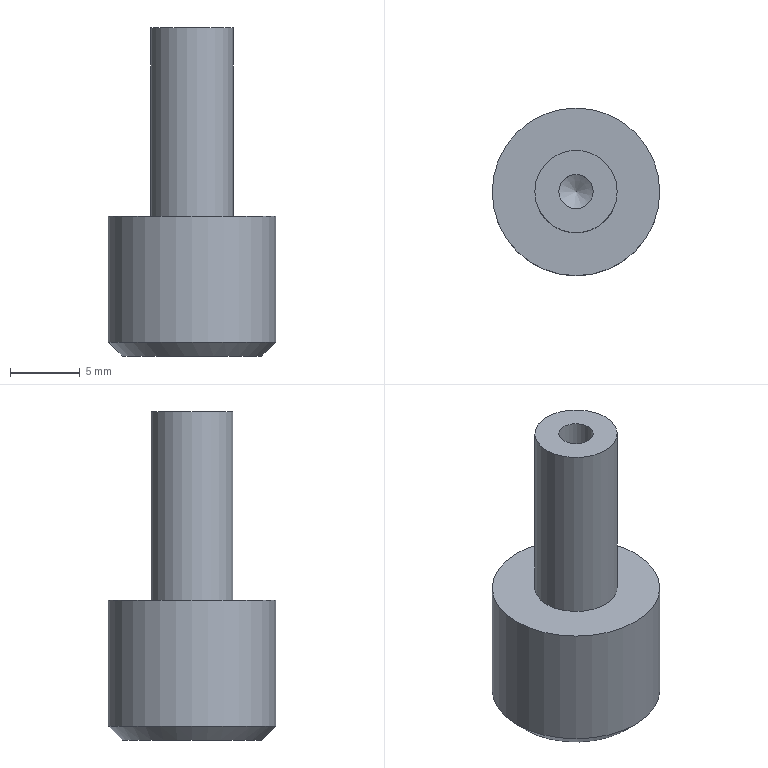Part | STEP file | 1-S938U-100524-007 | 1 solid | 10 faces | box 12 x 12 x 23.5 mm | volume 1339 mm3 | cylinder 4 | cone 3 | plane 3 | commonest cylinder face diameters 2.459 x1 3.242 x1 5.9 x1 12 x1
STEP:
#1=CARTESIAN_POINT('',(-6.,0.,1.));
#2=VERTEX_POINT('',#1);
#3=CARTESIAN_POINT('',(6.,0.,1.));
#4=VERTEX_POINT('',#3);
#5=CARTESIAN_POINT('',(0.,0.,1.));
#6=DIRECTION('',(0.,0.,-1.));
#7=DIRECTION('',(-1.,0.,0.));
#8=AXIS2_PLACEMENT_3D('',#5,#6,#7);
#9=CIRCLE('',#8,6.);
#10=EDGE_CURVE('',#2,#4,#9,.T.);
#11=ORIENTED_EDGE('',*,*,#10,.T.);
#12=CARTESIAN_POINT('',(5.,0.,0.));
#13=VERTEX_POINT('',#12);
#14=CARTESIAN_POINT('',(5.5,0.,0.5));
#15=DIRECTION('',(-0.7071,0.,-0.7071));
#16=VECTOR('',#15,5.5);
#17=LINE('',#14,#16);
#18=EDGE_CURVE('',#4,#13,#17,.T.);
#19=ORIENTED_EDGE('',*,*,#18,.T.);
#20=CARTESIAN_POINT('',(0.,0.,0.));
#21=DIRECTION('',(0.,0.,1.));
#22=DIRECTION('',(-1.,0.,0.));
#23=AXIS2_PLACEMENT_3D('',#20,#21,#22);
#24=CIRCLE('',#23,5.);
#25=EDGE_CURVE('',#13,#13,#24,.T.);
#26=ORIENTED_EDGE('',*,*,#25,.T.);
#27=ORIENTED_EDGE('',*,*,#18,.F.);
#28=CARTESIAN_POINT('',(0.,0.,1.));
#29=DIRECTION('',(0.,0.,-1.));
#30=DIRECTION('',(-1.,0.,0.));
#31=AXIS2_PLACEMENT_3D('',#28,#29,#30);
#32=CIRCLE('',#31,6.);
#33=EDGE_CURVE('',#4,#2,#32,.T.);
#34=ORIENTED_EDGE('',*,*,#33,.T.);
#35=EDGE_LOOP('',(#11,#19,#26,#27,#34));
#36=FACE_OUTER_BOUND('',#35,.T.);
#37=CARTESIAN_POINT('',(0.,0.,0.5));
#38=DIRECTION('',(0.,0.,1.));
#39=DIRECTION('',(-1.,0.,0.));
#40=AXIS2_PLACEMENT_3D('',#37,#38,#39);
#41=CONICAL_SURFACE('',#40,5.5,0.7854);
#42=ADVANCED_FACE('',(#36),#41,.T.);
#43=CARTESIAN_POINT('',(6.,0.,10.));
#44=VERTEX_POINT('',#43);
#45=CARTESIAN_POINT('',(-6.,0.,10.));
#46=VERTEX_POINT('',#45);
#47=CARTESIAN_POINT('',(0.,0.,10.));
#48=DIRECTION('',(0.,0.,1.));
#49=DIRECTION('',(1.,0.,0.));
#50=AXIS2_PLACEMENT_3D('',#47,#48,#49);
#51=CIRCLE('',#50,6.);
#52=EDGE_CURVE('',#44,#46,#51,.T.);
#53=ORIENTED_EDGE('',*,*,#52,.F.);
#54=CARTESIAN_POINT('',(0.,0.,10.));
#55=DIRECTION('',(0.,0.,1.));
#56=DIRECTION('',(1.,0.,0.));
#57=AXIS2_PLACEMENT_3D('',#54,#55,#56);
#58=CIRCLE('',#57,6.);
#59=EDGE_CURVE('',#46,#44,#58,.T.);
#60=ORIENTED_EDGE('',*,*,#59,.F.);
#61=CARTESIAN_POINT('',(-6.,0.,0.));
#62=DIRECTION('',(0.,0.,-1.));
#63=VECTOR('',#62,6.);
#64=LINE('',#61,#63);
#65=EDGE_CURVE('',#46,#2,#64,.T.);
#66=ORIENTED_EDGE('',*,*,#65,.T.);
#67=ORIENTED_EDGE('',*,*,#33,.F.);
#68=ORIENTED_EDGE('',*,*,#10,.F.);
#69=ORIENTED_EDGE('',*,*,#65,.F.);
#70=EDGE_LOOP('',(#53,#60,#66,#67,#68,#69));
#71=FACE_OUTER_BOUND('',#70,.T.);
#72=CARTESIAN_POINT('',(0.,0.,0.));
#73=DIRECTION('',(0.,0.,1.));
#74=DIRECTION('',(1.,0.,0.));
#75=AXIS2_PLACEMENT_3D('',#72,#73,#74);
#76=CYLINDRICAL_SURFACE('',#75,6.);
#77=ADVANCED_FACE('',(#71),#76,.T.);
#78=ORIENTED_EDGE('',*,*,#25,.F.);
#79=EDGE_LOOP('',(#78));
#80=FACE_OUTER_BOUND('',#79,.T.);
#81=CARTESIAN_POINT('',(-1.621,0.,0.));
#82=VERTEX_POINT('',#81);
#83=CARTESIAN_POINT('',(1.621,0.,0.));
#84=VERTEX_POINT('',#83);
#85=CARTESIAN_POINT('',(0.,0.,0.));
#86=DIRECTION('',(0.,0.,1.));
#87=DIRECTION('',(-1.,0.,0.));
#88=AXIS2_PLACEMENT_3D('',#85,#86,#87);
#89=CIRCLE('',#88,1.621);
#90=EDGE_CURVE('',#82,#84,#89,.T.);
#91=ORIENTED_EDGE('',*,*,#90,.T.);
#92=CARTESIAN_POINT('',(0.,0.,0.));
#93=DIRECTION('',(0.,0.,1.));
#94=DIRECTION('',(-1.,0.,0.));
#95=AXIS2_PLACEMENT_3D('',#92,#93,#94);
#96=CIRCLE('',#95,1.621);
#97=EDGE_CURVE('',#84,#82,#96,.T.);
#98=ORIENTED_EDGE('',*,*,#97,.T.);
#99=EDGE_LOOP('',(#91,#98));
#100=FACE_BOUND('',#99,.T.);
#101=CARTESIAN_POINT('',(0.,0.,0.));
#102=DIRECTION('',(0.,0.,1.));
#103=DIRECTION('',(1.,0.,0.));
#104=AXIS2_PLACEMENT_3D('',#101,#102,#103);
#105=PLANE('',#104);
#106=ADVANCED_FACE('',(#80,#100),#105,.F.);
#107=CARTESIAN_POINT('',(0.,0.,12.774));
#108=VERTEX_POINT('',#107);
#109=CARTESIAN_POINT('',(1.621,0.,11.8));
#110=VERTEX_POINT('',#109);
#111=CARTESIAN_POINT('',(0.8105,0.,12.287));
#112=DIRECTION('',(0.8572,0.,-0.515));
#113=VECTOR('',#112,0.8105);
#114=LINE('',#111,#113);
#115=EDGE_CURVE('',#108,#110,#114,.T.);
#116=ORIENTED_EDGE('',*,*,#115,.T.);
#117=CARTESIAN_POINT('',(-1.621,0.,11.8));
#118=VERTEX_POINT('',#117);
#119=CARTESIAN_POINT('',(0.,0.,11.8));
#120=DIRECTION('',(0.,0.,-1.));
#121=DIRECTION('',(-1.,0.,0.));
#122=AXIS2_PLACEMENT_3D('',#119,#120,#121);
#123=CIRCLE('',#122,1.621);
#124=EDGE_CURVE('',#110,#118,#123,.T.);
#125=ORIENTED_EDGE('',*,*,#124,.T.);
#126=CARTESIAN_POINT('',(0.,0.,11.8));
#127=DIRECTION('',(0.,0.,-1.));
#128=DIRECTION('',(-1.,0.,0.));
#129=AXIS2_PLACEMENT_3D('',#126,#127,#128);
#130=CIRCLE('',#129,1.621);
#131=EDGE_CURVE('',#118,#110,#130,.T.);
#132=ORIENTED_EDGE('',*,*,#131,.T.);
#133=ORIENTED_EDGE('',*,*,#115,.F.);
#134=EDGE_LOOP('',(#116,#125,#132,#133));
#135=FACE_OUTER_BOUND('',#134,.T.);
#136=CARTESIAN_POINT('',(0.,0.,12.287));
#137=DIRECTION('',(0.,0.,-1.));
#138=DIRECTION('',(-1.,0.,0.));
#139=AXIS2_PLACEMENT_3D('',#136,#137,#138);
#140=CONICAL_SURFACE('',#139,0.8105,1.03);
#141=ADVANCED_FACE('',(#135),#140,.F.);
#142=ORIENTED_EDGE('',*,*,#131,.F.);
#143=ORIENTED_EDGE('',*,*,#124,.F.);
#144=CARTESIAN_POINT('',(1.621,0.,5.9));
#145=DIRECTION('',(0.,0.,-1.));
#146=VECTOR('',#145,1.621);
#147=LINE('',#144,#146);
#148=EDGE_CURVE('',#110,#84,#147,.T.);
#149=ORIENTED_EDGE('',*,*,#148,.T.);
#150=ORIENTED_EDGE('',*,*,#90,.F.);
#151=ORIENTED_EDGE('',*,*,#97,.F.);
#152=ORIENTED_EDGE('',*,*,#148,.F.);
#153=EDGE_LOOP('',(#142,#143,#149,#150,#151,#152));
#154=FACE_OUTER_BOUND('',#153,.T.);
#155=CARTESIAN_POINT('',(0.,0.,5.9));
#156=DIRECTION('',(0.,0.,-1.));
#157=DIRECTION('',(-1.,0.,0.));
#158=AXIS2_PLACEMENT_3D('',#155,#156,#157);
#159=CYLINDRICAL_SURFACE('',#158,1.621);
#160=ADVANCED_FACE('',(#154),#159,.F.);
#161=CARTESIAN_POINT('',(0.,0.,13.961));
#162=VERTEX_POINT('',#161);
#163=CARTESIAN_POINT('',(-1.23,0.,14.7));
#164=VERTEX_POINT('',#163);
#165=CARTESIAN_POINT('',(-0.6148,0.,14.331));
#166=DIRECTION('',(-0.8572,0.,0.515));
#167=VECTOR('',#166,0.6148);
#168=LINE('',#165,#167);
#169=EDGE_CURVE('',#162,#164,#168,.T.);
#170=ORIENTED_EDGE('',*,*,#169,.T.);
#171=CARTESIAN_POINT('',(1.23,0.,14.7));
#172=VERTEX_POINT('',#171);
#173=CARTESIAN_POINT('',(0.,0.,14.7));
#174=DIRECTION('',(0.,0.,1.));
#175=DIRECTION('',(1.,0.,0.));
#176=AXIS2_PLACEMENT_3D('',#173,#174,#175);
#177=CIRCLE('',#176,1.23);
#178=EDGE_CURVE('',#164,#172,#177,.T.);
#179=ORIENTED_EDGE('',*,*,#178,.T.);
#180=CARTESIAN_POINT('',(0.,0.,14.7));
#181=DIRECTION('',(0.,0.,1.));
#182=DIRECTION('',(1.,0.,0.));
#183=AXIS2_PLACEMENT_3D('',#180,#181,#182);
#184=CIRCLE('',#183,1.23);
#185=EDGE_CURVE('',#172,#164,#184,.T.);
#186=ORIENTED_EDGE('',*,*,#185,.T.);
#187=ORIENTED_EDGE('',*,*,#169,.F.);
#188=EDGE_LOOP('',(#170,#179,#186,#187));
#189=FACE_OUTER_BOUND('',#188,.T.);
#190=CARTESIAN_POINT('',(0.,0.,14.331));
#191=DIRECTION('',(0.,0.,1.));
#192=DIRECTION('',(1.,0.,0.));
#193=AXIS2_PLACEMENT_3D('',#190,#191,#192);
#194=CONICAL_SURFACE('',#193,0.6148,1.03);
#195=ADVANCED_FACE('',(#189),#194,.F.);
#196=ORIENTED_EDGE('',*,*,#185,.F.);
#197=ORIENTED_EDGE('',*,*,#178,.F.);
#198=CARTESIAN_POINT('',(-1.23,0.,23.5));
#199=VERTEX_POINT('',#198);
#200=CARTESIAN_POINT('',(-1.23,0.,19.1));
#201=DIRECTION('',(0.,0.,1.));
#202=VECTOR('',#201,1.23);
#203=LINE('',#200,#202);
#204=EDGE_CURVE('',#164,#199,#203,.T.);
#205=ORIENTED_EDGE('',*,*,#204,.T.);
#206=CARTESIAN_POINT('',(1.23,0.,23.5));
#207=VERTEX_POINT('',#206);
#208=CARTESIAN_POINT('',(0.,0.,23.5));
#209=DIRECTION('',(0.,0.,-1.));
#210=DIRECTION('',(1.,0.,0.));
#211=AXIS2_PLACEMENT_3D('',#208,#209,#210);
#212=CIRCLE('',#211,1.23);
#213=EDGE_CURVE('',#207,#199,#212,.T.);
#214=ORIENTED_EDGE('',*,*,#213,.F.);
#215=CARTESIAN_POINT('',(0.,0.,23.5));
#216=DIRECTION('',(0.,0.,-1.));
#217=DIRECTION('',(1.,0.,0.));
#218=AXIS2_PLACEMENT_3D('',#215,#216,#217);
#219=CIRCLE('',#218,1.23);
#220=EDGE_CURVE('',#199,#207,#219,.T.);
#221=ORIENTED_EDGE('',*,*,#220,.F.);
#222=ORIENTED_EDGE('',*,*,#204,.F.);
#223=EDGE_LOOP('',(#196,#197,#205,#214,#221,#222));
#224=FACE_OUTER_BOUND('',#223,.T.);
#225=CARTESIAN_POINT('',(0.,0.,19.1));
#226=DIRECTION('',(0.,0.,1.));
#227=DIRECTION('',(1.,0.,0.));
#228=AXIS2_PLACEMENT_3D('',#225,#226,#227);
#229=CYLINDRICAL_SURFACE('',#228,1.23);
#230=ADVANCED_FACE('',(#224),#229,.F.);
#231=CARTESIAN_POINT('',(2.95,0.,23.5));
#232=VERTEX_POINT('',#231);
#233=CARTESIAN_POINT('',(-2.95,0.,23.5));
#234=VERTEX_POINT('',#233);
#235=CARTESIAN_POINT('',(0.,0.,23.5));
#236=DIRECTION('',(0.,0.,1.));
#237=DIRECTION('',(1.,0.,0.));
#238=AXIS2_PLACEMENT_3D('',#235,#236,#237);
#239=CIRCLE('',#238,2.95);
#240=EDGE_CURVE('',#232,#234,#239,.T.);
#241=ORIENTED_EDGE('',*,*,#240,.F.);
#242=CARTESIAN_POINT('',(0.,0.,23.5));
#243=DIRECTION('',(0.,0.,1.));
#244=DIRECTION('',(1.,0.,0.));
#245=AXIS2_PLACEMENT_3D('',#242,#243,#244);
#246=CIRCLE('',#245,2.95);
#247=EDGE_CURVE('',#234,#232,#246,.T.);
#248=ORIENTED_EDGE('',*,*,#247,.F.);
#249=CARTESIAN_POINT('',(-2.95,0.,10.));
#250=VERTEX_POINT('',#249);
#251=CARTESIAN_POINT('',(-2.95,0.,10.));
#252=DIRECTION('',(0.,0.,-1.));
#253=VECTOR('',#252,2.95);
#254=LINE('',#251,#253);
#255=EDGE_CURVE('',#234,#250,#254,.T.);
#256=ORIENTED_EDGE('',*,*,#255,.T.);
#257=CARTESIAN_POINT('',(2.95,0.,10.));
#258=VERTEX_POINT('',#257);
#259=CARTESIAN_POINT('',(0.,0.,10.));
#260=DIRECTION('',(0.,0.,-1.));
#261=DIRECTION('',(1.,0.,0.));
#262=AXIS2_PLACEMENT_3D('',#259,#260,#261);
#263=CIRCLE('',#262,2.95);
#264=EDGE_CURVE('',#258,#250,#263,.T.);
#265=ORIENTED_EDGE('',*,*,#264,.F.);
#266=CARTESIAN_POINT('',(0.,0.,10.));
#267=DIRECTION('',(0.,0.,-1.));
#268=DIRECTION('',(1.,0.,0.));
#269=AXIS2_PLACEMENT_3D('',#266,#267,#268);
#270=CIRCLE('',#269,2.95);
#271=EDGE_CURVE('',#250,#258,#270,.T.);
#272=ORIENTED_EDGE('',*,*,#271,.F.);
#273=ORIENTED_EDGE('',*,*,#255,.F.);
#274=EDGE_LOOP('',(#241,#248,#256,#265,#272,#273));
#275=FACE_OUTER_BOUND('',#274,.T.);
#276=CARTESIAN_POINT('',(0.,0.,10.));
#277=DIRECTION('',(0.,0.,1.));
#278=DIRECTION('',(1.,0.,0.));
#279=AXIS2_PLACEMENT_3D('',#276,#277,#278);
#280=CYLINDRICAL_SURFACE('',#279,2.95);
#281=ADVANCED_FACE('',(#275),#280,.T.);
#282=ORIENTED_EDGE('',*,*,#240,.T.);
#283=ORIENTED_EDGE('',*,*,#247,.T.);
#284=EDGE_LOOP('',(#282,#283));
#285=FACE_OUTER_BOUND('',#284,.T.);
#286=ORIENTED_EDGE('',*,*,#213,.T.);
#287=ORIENTED_EDGE('',*,*,#220,.T.);
#288=EDGE_LOOP('',(#286,#287));
#289=FACE_BOUND('',#288,.T.);
#290=CARTESIAN_POINT('',(0.,0.,23.5));
#291=DIRECTION('',(0.,0.,1.));
#292=DIRECTION('',(1.,0.,0.));
#293=AXIS2_PLACEMENT_3D('',#290,#291,#292);
#294=PLANE('',#293);
#295=ADVANCED_FACE('',(#285,#289),#294,.T.);
#296=ORIENTED_EDGE('',*,*,#52,.T.);
#297=ORIENTED_EDGE('',*,*,#59,.T.);
#298=EDGE_LOOP('',(#296,#297));
#299=FACE_OUTER_BOUND('',#298,.T.);
#300=ORIENTED_EDGE('',*,*,#264,.T.);
#301=ORIENTED_EDGE('',*,*,#271,.T.);
#302=EDGE_LOOP('',(#300,#301));
#303=FACE_BOUND('',#302,.T.);
#304=CARTESIAN_POINT('',(0.,0.,10.));
#305=DIRECTION('',(0.,0.,1.));
#306=DIRECTION('',(1.,0.,0.));
#307=AXIS2_PLACEMENT_3D('',#304,#305,#306);
#308=PLANE('',#307);
#309=ADVANCED_FACE('',(#299,#303),#308,.T.);
#310=CLOSED_SHELL('',(#42,#77,#106,#141,#160,#195,#230,#281,#295,#309));
#311=MANIFOLD_SOLID_BREP('',#310);
#312=(LENGTH_UNIT()NAMED_UNIT(*)SI_UNIT(.MILLI.,.METRE.));
#313=UNCERTAINTY_MEASURE_WITH_UNIT(LENGTH_MEASURE(0.01),#312,'','');
#314=(NAMED_UNIT(*)PLANE_ANGLE_UNIT()SI_UNIT($,.RADIAN.));
#315=(NAMED_UNIT(*)SI_UNIT($,.STERADIAN.)SOLID_ANGLE_UNIT());
#316=(GEOMETRIC_REPRESENTATION_CONTEXT(3)GLOBAL_UNCERTAINTY_ASSIGNED_CONTEXT((#313))GLOBAL_UNIT_ASSIGNED_CONTEXT((#312,#314,#315))REPRESENTATION_CONTEXT('',''));
#317=ADVANCED_BREP_SHAPE_REPRESENTATION('',(#311),#316);